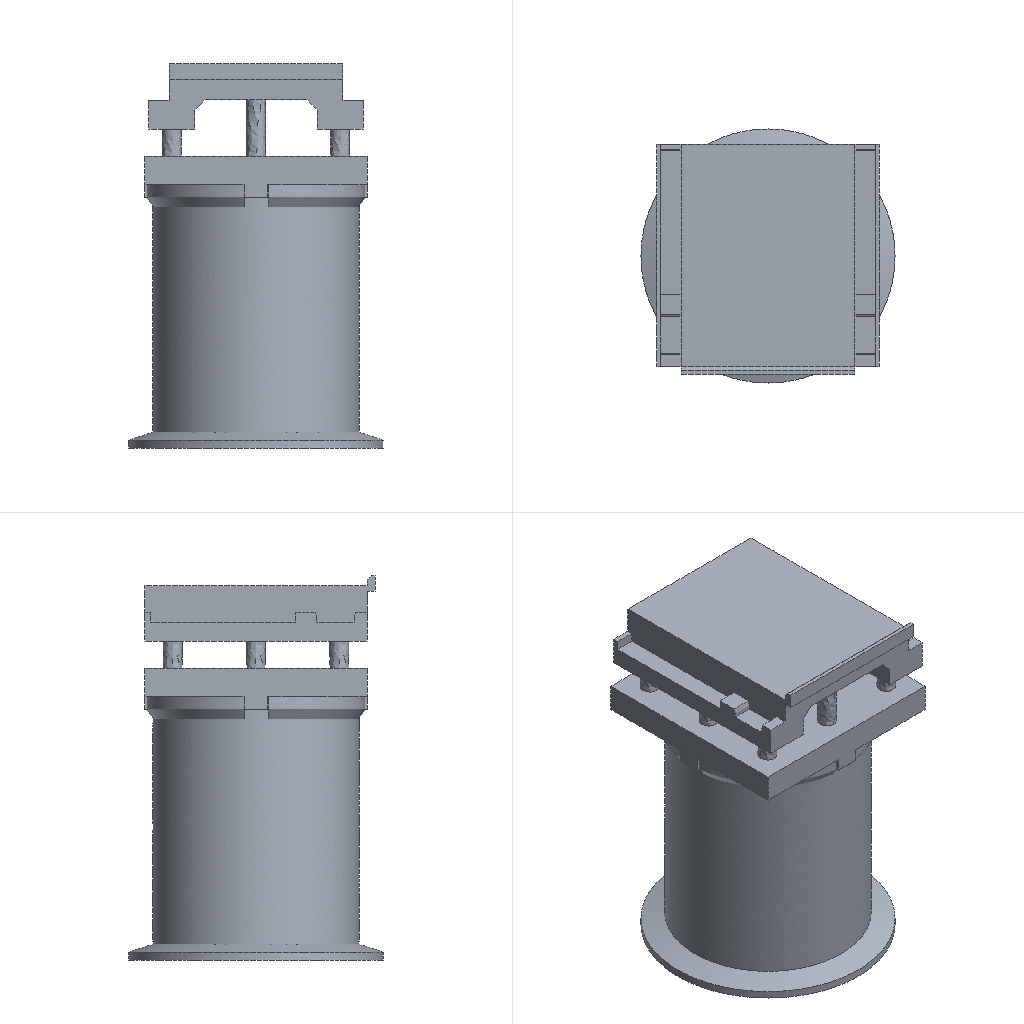Simulation study | ansys workbench
Ansys APDL input file, long lists of numbers shortened:
/batch
/config,noeldb,1     ! force off writing results to database
*get,_wallstrt,active,,time,wall
! ANSYS input file written by Workbench version 2022 R1
! File used for geometry attach:
/title,___--____ 3 (C5)
! ****** Begin Custom Load Command Snippet ******
/COM, ACT Extensions:
/COM,     LSDYNA, 2021.1
/COM,
! ****** End   Custom Load Command Snippet ******
*DIM,_wb_ProjectScratch_dir,string,248
_wb_ProjectScratch_dir(1) = ''
*DIM,_wb_SolverFiles_dir,string,248
_wb_SolverFiles_dir(1) = ''
*DIM,_wb_userfiles_dir,string,248
_wb_userfiles_dir(1) = ''
/com,--- Data in consistent MKS units. See Solving Units in the help system for more information.
/units,MKS
/nopr
/wb,file,start              !  signify a WB generated input file
/prep7
! Turn off shape checking because checks already performed inside WB mesher.
! See help system for more information.
SHPP,OFF,,NOWARN
/nolist
etcon,set             ! allow ANSYS to choose best KEYOP's for 180x elements, resets any applicable keyopt to MAPDL defaults
/com,*********** Nodes for the whole assembly ***********
nblock,3,,165333
(1i9,3e20.9e3)
        1    -4.091861413E+02     3.968814041E+01    -2.039000000E+01
! (150302 more lines like these left out)
-1
/wb,elem,start            !  set before creation of elements
/com,*********** Elements for Body 1 "a953f0-7" ***********
et,1,187
eblock,19,solid,,87505
(19i9)
        1        1        1        1        0        0        0        0       10        0        1    11820    23372    11975    23358    91085    91919    91082    91084
! (175009 more lines like these left out)
-1
/wb,elem,end               !  done creating elements
/com,*********** Send User Defined Coordinate System(s) ***********
csys,0
toffst,273.15,  ! Temperature offset from absolute zero
/com,*********** Set Reference Temperature ***********
tref,22.
/wb,mat,start              !  starting to send materials
/com,*********** Send Materials ***********
Temperature = 'TEMP' ! Temperature
MP,DENS,1,2300,	! kg m^-3
MP,ALPX,1,1.4e-05,	! C^-1
MP,C,1,780,	! J kg^-1 C^-1
MP,KXX,1,0.72,	! W m^-1 C^-1
MP,EX,1,30000000000,	! Pa
MP,NUXY,1,0.18,
/wb,mat,end                !  done sending materials
!************************* Model Summary ********************
!a953f0-7,	混凝土,	matid,	1
!************************* End Model Summary ********************
! get the diagonal of the bounding box. Needed later for other things
*get,_xmin,node,,mnloc,x
*get,_ymin,node,,mnloc,y
*get,_zmin,node,,mnloc,z
*get,_xmax,node,,mxloc,x
*get,_ymax,node,,mxloc,y
*get,_zmax,node,,mxloc,z
_ASMDIAG=(_xmax-_xmin)*(_xmax-_xmin)+(_ymax-_ymin)*(_ymax-_ymin)+(_zmax-_zmin)*(_zmax-_zmin)
_ASMDIAG=SQRT(_ASMDIAG)
/wb,contact,start          !  starting to send contact
/wb,contact,end            !  done creating contacts
/golist
/wb,load,start             !  starting to send loads
/com,*********** Fixed Supports ***********
CMBLOCK,_FIXEDSU,NODE,     7355
(8i10)
         1        96       121       122       123       124       125       126
! (919 more lines like these left out)
cmsel,s,_FIXEDSU
d,all,all
nsel,all
/com,*********** Define Force Using Surface Effect Elements ***********
local,12,0,0.,0.,0.,0.,0.,0.
csys,0
et,2,154
eblock,10,,,7449
(15i9)
   119600        2        2        2       12        4        3     5956     5956    23385    23389     5956    23396
! (7448 more lines like these left out)
-1
esel,s,type,,2
keyop,2,2,1                ! Apply load in local coordinate system
keyop,2,7,1                ! Use original area so load is constant in large deformation
esel,all
/gst,on,on
fini
*get,_numnode,node,0,count
*get,_numelem,elem,0,count
*get, _MAXELEMNUM, elem, 0, NUM, MAX
*get, _MAXNODENUM, node, 0, NUM, MAX
*get, _MAXELEMTYPE, etyp, 0, NUM, MAX
*get, _MAXREALCONST, real, 0, NUM, MAX
/go
/wb,load,end               !  done creating loads
/com,--- Number of total nodes = %_numnode%
/com,--- Number of contact elements = 7449
/com,--- Number of spring elements = 0
/com,--- Number of bearing elements = 0
/com,--- Number of solid elements = 87505
/com,--- Number of condensed parts = 0
/com,--- Number of total elements = %_numelem%
*get,_wallbsol,active,,time,wall
/com,****************************************************************************
/com,*************************    SOLUTION       ********************************
/com,****************************************************************************
/solu
antype,0                   ! static analysis
_thickRatio=  1     ! Ratio of thick parts in the model
eqsl,pcg,1e-8,,,,,,1
cntr,print,1               ! print out contact info and also make no initial contact an error
dmpoption,emat,no             ! Don't combine emat file for DANSYS
dmpoption,esav,no             ! Don't combine esav file for DANSYS
nldiag,cont,iter           ! print out contact info each equilibrium iteration
rescontrol,,none                 ! Do not keep any restart files
/com,****************************************************
/com,******************* SOLVE FOR LS 1 OF 1 ****************
esel,s,type,,2
nsle
sfe,all,1,pres,1,0.
sfe,all,2,pres,1,-1170.24
sfe,all,3,pres,1,0.
nsel,all
esel,all
acel,0.,0.,9.807
/nopr
/gopr
nsub,1,1,1
time,1.
outres,erase
outres,all,none
outres,nsol,all,
outres,rsol,all
outres,eangl,all
outres,etmp,all
outres,veng,all
outres,strs,all,
outres,epel,all,
outres,eppl,all,
outres,cont,all,
! *********** WB SOLVE COMMAND ***********
! check interactive state
*get,ANSINTER_,active,,int
*if,ANSINTER_,ne,0,then
/eof
*endif
solve
/com *************** Write FE CONNECTORS *********
CEWRITE,file,ce,,INTE
/com,****************************************************
/com,*************** FINISHED SOLVE FOR LS 1 *************
*get,_wallasol,active,,time,wall
/nopr
*get,_numnode,node,0,count
*get,_numelem,elem,0,count
*get, _MAXELEMNUM, elem, 0, NUM, MAX
*get, _MAXNODENUM, node, 0, NUM, MAX,,,INTERNAL
*get, _MAXELEMTYPE, etyp, 0, NUM, MAX
*get, _MAXREALCONST, real, 0, NUM, MAX
/gopr
*get,_PCGITER,active,,solu,cgiter
/post1
xmlo,ENCODING,ISO-8859-1
xmlo,parm
/xml,parm,xml
fini
/gopr
*get,_walldone,active,,time,wall
_preptime=(_wallbsol-_wallstrt)*3600
_solvtime=(_wallasol-_wallbsol)*3600
_posttime=(_walldone-_wallasol)*3600
_totaltim=(_walldone-_wallstrt)*3600
*get,_dlbratio,active,0,solu,dlbr
*get,_combtime,active,0,solu,comb
*get,_ssmode,active,0,solu,ssmm
*get,_ndofs,active,0,solu,ndof
*get,_sol_end_time,active,0,set,time
*if,_sol_end_time,eq,1.,then
/fclean				!clean distributed files
*endif
/com,--- Total number of nodes = %_numnode%
/com,--- Total number of elements = %_numelem%
/com,--- Element load balance ratio = %_dlbratio%
/com,--- Time to combine distributed files = %_combtime%
/com,--- Sparse memory mode = %_ssmode%
/com,--- Number of DOF = %_ndofs%
/wb,file,end               ! done with WB generated input